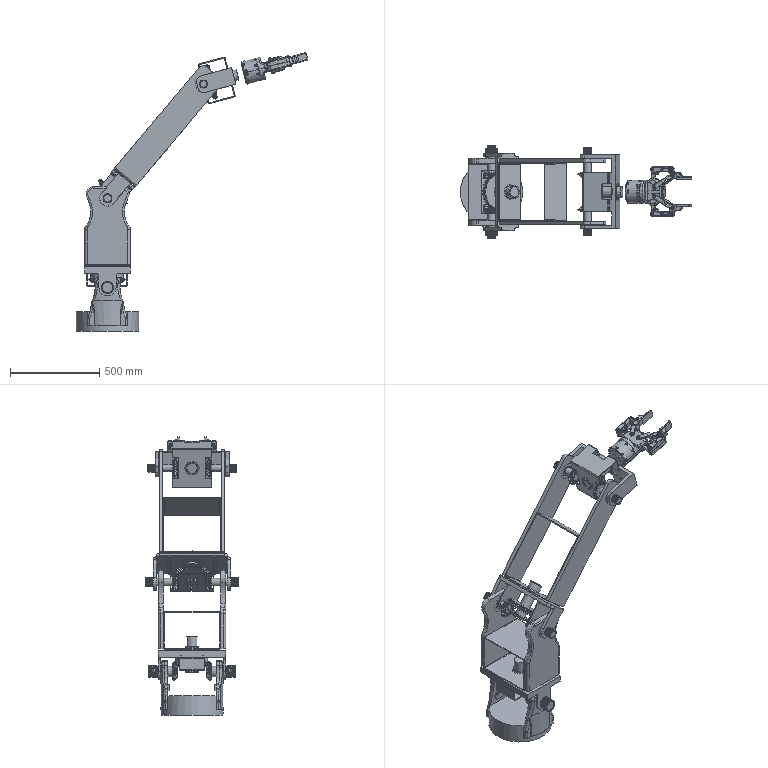Part | NX | features BREP 1 | 130 solids | 8552 faces | volume 42296418 mm3 | spline 2578 | plane 2574 | cylinder 2351 | cone 923 | torus 126 | commonest cylinder face diameters 4 x341 5 x284 8 x179 10 x170 0.508 x96 16 x82